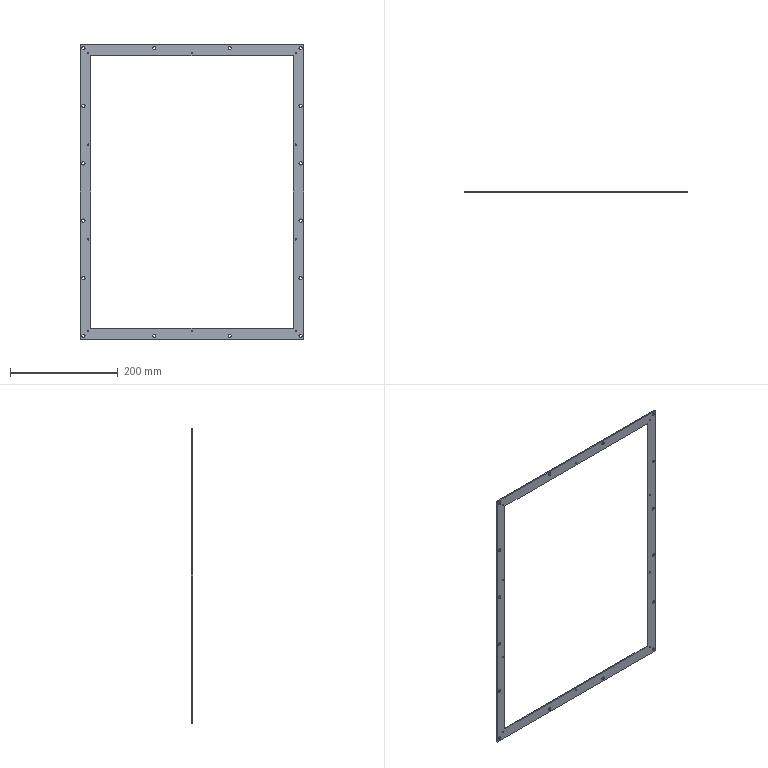Part | NX | features solid 2 | 1 solid | 62 faces | box 415 x 2 x 546 mm | volume 72680 mm3 | cylinder 52 | plane 10 | commonest cylinder face diameters 6 x32 2.459 x20